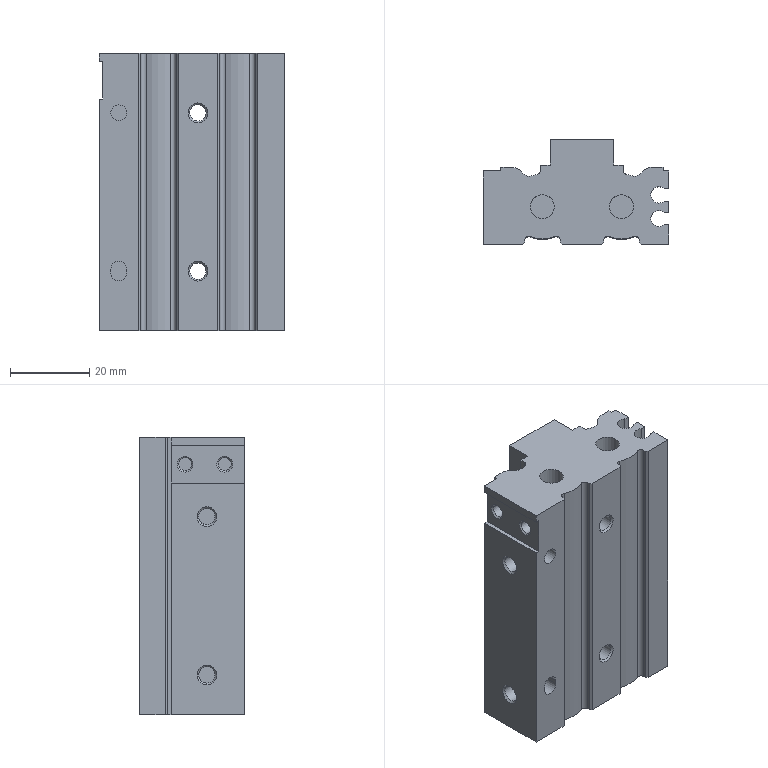Part | NX | 1 solid | 109 faces | box 47 x 26.5 x 70 mm | volume 57009 mm3 | plane 60 | cylinder 39 | cone 10 | commonest cylinder face diameters 2 x6 3.242 x6 4 x5 4.134 x4 4.2 x4 16.4 x4